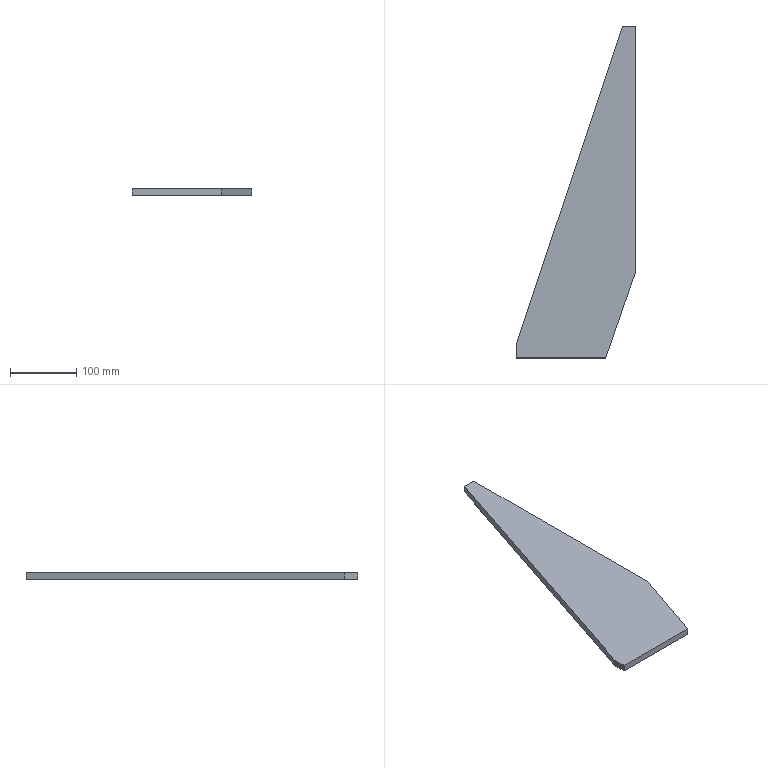Part | SolidWorks | features Extrusion 1 | 1 solid | 8 faces | box 180 x 500 x 10 mm | volume 486750 mm3 | plane 8
STEP:
#1=CARTESIAN_POINT('',(-45.,0.,-5.));
#2=VERTEX_POINT('',#1);
#3=CARTESIAN_POINT('',(0.,130.,-5.));
#4=VERTEX_POINT('',#3);
#5=CARTESIAN_POINT('',(-45.,0.,-5.));
#6=DIRECTION('',(0.3271,0.945,0.));
#7=VECTOR('',#6,1000.);
#8=LINE('',#5,#7);
#9=EDGE_CURVE('',#2,#4,#8,.T.);
#10=ORIENTED_EDGE('',*,*,#9,.T.);
#11=CARTESIAN_POINT('',(0.,130.,5.));
#12=VERTEX_POINT('',#11);
#13=CARTESIAN_POINT('',(0.,130.,5.));
#14=DIRECTION('',(0.,0.,-1.));
#15=VECTOR('',#14,1000.);
#16=LINE('',#13,#15);
#17=EDGE_CURVE('',#12,#4,#16,.T.);
#18=ORIENTED_EDGE('',*,*,#17,.F.);
#19=CARTESIAN_POINT('',(-45.,0.,5.));
#20=VERTEX_POINT('',#19);
#21=CARTESIAN_POINT('',(-45.,0.,5.));
#22=DIRECTION('',(0.3271,0.945,0.));
#23=VECTOR('',#22,1000.);
#24=LINE('',#21,#23);
#25=EDGE_CURVE('',#20,#12,#24,.T.);
#26=ORIENTED_EDGE('',*,*,#25,.F.);
#27=CARTESIAN_POINT('',(-45.,0.,5.));
#28=DIRECTION('',(0.,0.,-1.));
#29=VECTOR('',#28,1000.);
#30=LINE('',#27,#29);
#31=EDGE_CURVE('',#20,#2,#30,.T.);
#32=ORIENTED_EDGE('',*,*,#31,.T.);
#33=EDGE_LOOP('',(#10,#18,#26,#32));
#34=FACE_OUTER_BOUND('',#33,.T.);
#35=CARTESIAN_POINT('',(-45.,0.,5.));
#36=DIRECTION('',(-0.945,0.3271,0.));
#37=DIRECTION('',(-0.3271,-0.945,0.));
#38=AXIS2_PLACEMENT_3D('',#35,#36,#37);
#39=PLANE('',#38);
#40=ADVANCED_FACE('',(#34),#39,.F.);
#41=CARTESIAN_POINT('',(0.,500.,-5.));
#42=VERTEX_POINT('',#41);
#43=CARTESIAN_POINT('',(0.,130.,-5.));
#44=DIRECTION('',(0.,1.,0.));
#45=VECTOR('',#44,1000.);
#46=LINE('',#43,#45);
#47=EDGE_CURVE('',#4,#42,#46,.T.);
#48=ORIENTED_EDGE('',*,*,#47,.T.);
#49=CARTESIAN_POINT('',(0.,500.,5.));
#50=VERTEX_POINT('',#49);
#51=CARTESIAN_POINT('',(0.,500.,5.));
#52=DIRECTION('',(0.,0.,-1.));
#53=VECTOR('',#52,1000.);
#54=LINE('',#51,#53);
#55=EDGE_CURVE('',#50,#42,#54,.T.);
#56=ORIENTED_EDGE('',*,*,#55,.F.);
#57=CARTESIAN_POINT('',(0.,130.,5.));
#58=DIRECTION('',(0.,1.,0.));
#59=VECTOR('',#58,1000.);
#60=LINE('',#57,#59);
#61=EDGE_CURVE('',#12,#50,#60,.T.);
#62=ORIENTED_EDGE('',*,*,#61,.F.);
#63=ORIENTED_EDGE('',*,*,#17,.T.);
#64=EDGE_LOOP('',(#48,#56,#62,#63));
#65=FACE_OUTER_BOUND('',#64,.T.);
#66=CARTESIAN_POINT('',(0.,130.,5.));
#67=DIRECTION('',(-1.,0.,0.));
#68=DIRECTION('',(0.,0.,1.));
#69=AXIS2_PLACEMENT_3D('',#66,#67,#68);
#70=PLANE('',#69);
#71=ADVANCED_FACE('',(#65),#70,.F.);
#72=CARTESIAN_POINT('',(-20.,500.,-5.));
#73=VERTEX_POINT('',#72);
#74=CARTESIAN_POINT('',(0.,500.,-5.));
#75=DIRECTION('',(-1.,0.,0.));
#76=VECTOR('',#75,1000.);
#77=LINE('',#74,#76);
#78=EDGE_CURVE('',#42,#73,#77,.T.);
#79=ORIENTED_EDGE('',*,*,#78,.T.);
#80=CARTESIAN_POINT('',(-20.,500.,5.));
#81=VERTEX_POINT('',#80);
#82=CARTESIAN_POINT('',(-20.,500.,5.));
#83=DIRECTION('',(0.,0.,-1.));
#84=VECTOR('',#83,1000.);
#85=LINE('',#82,#84);
#86=EDGE_CURVE('',#81,#73,#85,.T.);
#87=ORIENTED_EDGE('',*,*,#86,.F.);
#88=CARTESIAN_POINT('',(0.,500.,5.));
#89=DIRECTION('',(-1.,0.,0.));
#90=VECTOR('',#89,1000.);
#91=LINE('',#88,#90);
#92=EDGE_CURVE('',#50,#81,#91,.T.);
#93=ORIENTED_EDGE('',*,*,#92,.F.);
#94=ORIENTED_EDGE('',*,*,#55,.T.);
#95=EDGE_LOOP('',(#79,#87,#93,#94));
#96=FACE_OUTER_BOUND('',#95,.T.);
#97=CARTESIAN_POINT('',(0.,500.,5.));
#98=DIRECTION('',(0.,-1.,0.));
#99=DIRECTION('',(0.,0.,-1.));
#100=AXIS2_PLACEMENT_3D('',#97,#98,#99);
#101=PLANE('',#100);
#102=ADVANCED_FACE('',(#96),#101,.F.);
#103=CARTESIAN_POINT('',(-180.,20.,-5.));
#104=VERTEX_POINT('',#103);
#105=CARTESIAN_POINT('',(-20.,500.,-5.));
#106=DIRECTION('',(-0.3162,-0.9487,0.));
#107=VECTOR('',#106,1000.);
#108=LINE('',#105,#107);
#109=EDGE_CURVE('',#73,#104,#108,.T.);
#110=ORIENTED_EDGE('',*,*,#109,.T.);
#111=CARTESIAN_POINT('',(-180.,20.,5.));
#112=VERTEX_POINT('',#111);
#113=CARTESIAN_POINT('',(-180.,20.,5.));
#114=DIRECTION('',(0.,0.,-1.));
#115=VECTOR('',#114,1000.);
#116=LINE('',#113,#115);
#117=EDGE_CURVE('',#112,#104,#116,.T.);
#118=ORIENTED_EDGE('',*,*,#117,.F.);
#119=CARTESIAN_POINT('',(-20.,500.,5.));
#120=DIRECTION('',(-0.3162,-0.9487,0.));
#121=VECTOR('',#120,1000.);
#122=LINE('',#119,#121);
#123=EDGE_CURVE('',#81,#112,#122,.T.);
#124=ORIENTED_EDGE('',*,*,#123,.F.);
#125=ORIENTED_EDGE('',*,*,#86,.T.);
#126=EDGE_LOOP('',(#110,#118,#124,#125));
#127=FACE_OUTER_BOUND('',#126,.T.);
#128=CARTESIAN_POINT('',(-20.,500.,5.));
#129=DIRECTION('',(0.9487,-0.3162,0.));
#130=DIRECTION('',(0.3162,0.9487,0.));
#131=AXIS2_PLACEMENT_3D('',#128,#129,#130);
#132=PLANE('',#131);
#133=ADVANCED_FACE('',(#127),#132,.F.);
#134=CARTESIAN_POINT('',(-180.,0.,-5.));
#135=VERTEX_POINT('',#134);
#136=CARTESIAN_POINT('',(-180.,20.,-5.));
#137=DIRECTION('',(0.,-1.,0.));
#138=VECTOR('',#137,1000.);
#139=LINE('',#136,#138);
#140=EDGE_CURVE('',#104,#135,#139,.T.);
#141=ORIENTED_EDGE('',*,*,#140,.T.);
#142=CARTESIAN_POINT('',(-180.,0.,5.));
#143=VERTEX_POINT('',#142);
#144=CARTESIAN_POINT('',(-180.,0.,5.));
#145=DIRECTION('',(0.,0.,-1.));
#146=VECTOR('',#145,1000.);
#147=LINE('',#144,#146);
#148=EDGE_CURVE('',#143,#135,#147,.T.);
#149=ORIENTED_EDGE('',*,*,#148,.F.);
#150=CARTESIAN_POINT('',(-180.,20.,5.));
#151=DIRECTION('',(0.,-1.,0.));
#152=VECTOR('',#151,1000.);
#153=LINE('',#150,#152);
#154=EDGE_CURVE('',#112,#143,#153,.T.);
#155=ORIENTED_EDGE('',*,*,#154,.F.);
#156=ORIENTED_EDGE('',*,*,#117,.T.);
#157=EDGE_LOOP('',(#141,#149,#155,#156));
#158=FACE_OUTER_BOUND('',#157,.T.);
#159=CARTESIAN_POINT('',(-180.,20.,5.));
#160=DIRECTION('',(1.,0.,0.));
#161=DIRECTION('',(0.,0.,-1.));
#162=AXIS2_PLACEMENT_3D('',#159,#160,#161);
#163=PLANE('',#162);
#164=ADVANCED_FACE('',(#158),#163,.F.);
#165=CARTESIAN_POINT('',(-180.,0.,-5.));
#166=DIRECTION('',(1.,0.,0.));
#167=VECTOR('',#166,1000.);
#168=LINE('',#165,#167);
#169=EDGE_CURVE('',#135,#2,#168,.T.);
#170=ORIENTED_EDGE('',*,*,#169,.T.);
#171=ORIENTED_EDGE('',*,*,#31,.F.);
#172=CARTESIAN_POINT('',(-180.,0.,5.));
#173=DIRECTION('',(1.,0.,0.));
#174=VECTOR('',#173,1000.);
#175=LINE('',#172,#174);
#176=EDGE_CURVE('',#143,#20,#175,.T.);
#177=ORIENTED_EDGE('',*,*,#176,.F.);
#178=ORIENTED_EDGE('',*,*,#148,.T.);
#179=EDGE_LOOP('',(#170,#171,#177,#178));
#180=FACE_OUTER_BOUND('',#179,.T.);
#181=CARTESIAN_POINT('',(-180.,0.,5.));
#182=DIRECTION('',(0.,1.,0.));
#183=DIRECTION('',(0.,0.,1.));
#184=AXIS2_PLACEMENT_3D('',#181,#182,#183);
#185=PLANE('',#184);
#186=ADVANCED_FACE('',(#180),#185,.F.);
#187=ORIENTED_EDGE('',*,*,#25,.T.);
#188=ORIENTED_EDGE('',*,*,#61,.T.);
#189=ORIENTED_EDGE('',*,*,#92,.T.);
#190=ORIENTED_EDGE('',*,*,#123,.T.);
#191=ORIENTED_EDGE('',*,*,#154,.T.);
#192=ORIENTED_EDGE('',*,*,#176,.T.);
#193=EDGE_LOOP('',(#187,#188,#189,#190,#191,#192));
#194=FACE_OUTER_BOUND('',#193,.T.);
#195=CARTESIAN_POINT('',(128.077,500.,5.));
#196=DIRECTION('',(0.,0.,1.));
#197=DIRECTION('',(1.,0.,0.));
#198=AXIS2_PLACEMENT_3D('',#195,#196,#197);
#199=PLANE('',#198);
#200=ADVANCED_FACE('',(#194),#199,.T.);
#201=ORIENTED_EDGE('',*,*,#9,.F.);
#202=ORIENTED_EDGE('',*,*,#169,.F.);
#203=ORIENTED_EDGE('',*,*,#140,.F.);
#204=ORIENTED_EDGE('',*,*,#109,.F.);
#205=ORIENTED_EDGE('',*,*,#78,.F.);
#206=ORIENTED_EDGE('',*,*,#47,.F.);
#207=EDGE_LOOP('',(#201,#202,#203,#204,#205,#206));
#208=FACE_OUTER_BOUND('',#207,.T.);
#209=CARTESIAN_POINT('',(128.077,500.,-5.));
#210=DIRECTION('',(0.,0.,1.));
#211=DIRECTION('',(1.,0.,0.));
#212=AXIS2_PLACEMENT_3D('',#209,#210,#211);
#213=PLANE('',#212);
#214=ADVANCED_FACE('',(#208),#213,.F.);
#215=CLOSED_SHELL('',(#40,#71,#102,#133,#164,#186,#200,#214));
#216=MANIFOLD_SOLID_BREP('',#215);
#217=CARTESIAN_POINT('',(0.,0.,0.));
#218=DIRECTION('',(0.,0.,1.));
#219=DIRECTION('',(1.,0.,0.));
#220=AXIS2_PLACEMENT_3D('',#217,#218,#219);
#221=(LENGTH_UNIT()NAMED_UNIT(*)SI_UNIT(.MILLI.,.METRE.));
#222=UNCERTAINTY_MEASURE_WITH_UNIT(LENGTH_MEASURE(0.00001),#221,'','');
#223=(NAMED_UNIT(*)PLANE_ANGLE_UNIT()SI_UNIT($,.RADIAN.));
#224=(NAMED_UNIT(*)SI_UNIT($,.STERADIAN.)SOLID_ANGLE_UNIT());
#225=(GEOMETRIC_REPRESENTATION_CONTEXT(3)GLOBAL_UNCERTAINTY_ASSIGNED_CONTEXT((#222))GLOBAL_UNIT_ASSIGNED_CONTEXT((#221,#223,#224))REPRESENTATION_CONTEXT('',''));
#226=ADVANCED_BREP_SHAPE_REPRESENTATION('',(#216,#220),#225);